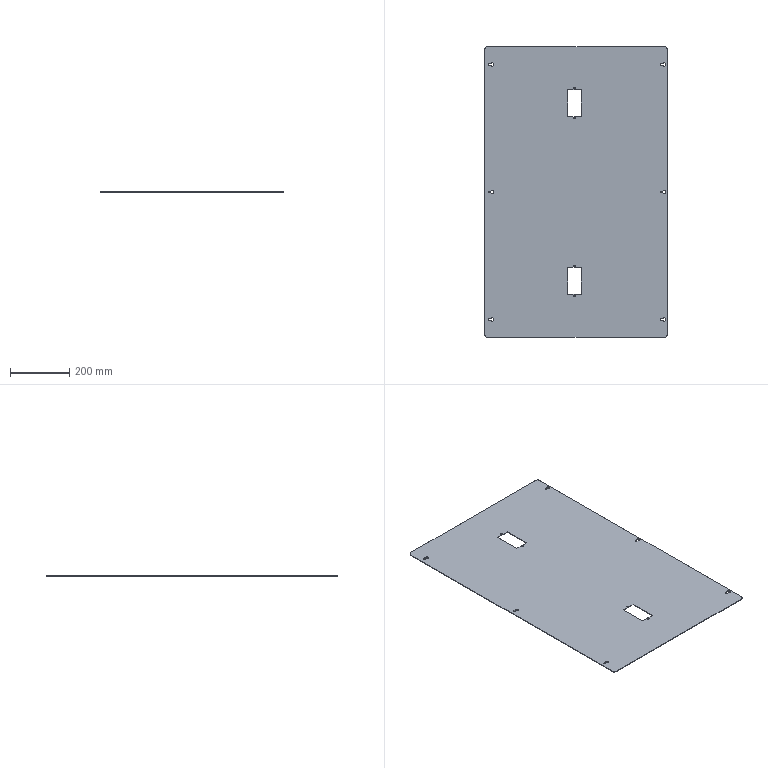Part | SolidWorks | features ICE 4, Extrusion 1, Fillet 1, LPattern 1 | 1 solid | 56 faces | box 615 x 980 x 2 mm | volume 1186991 mm3 | cylinder 30 | plane 26 | commonest cylinder face diameters 6.6 x12 4.5 x8 11 x6 20 x4